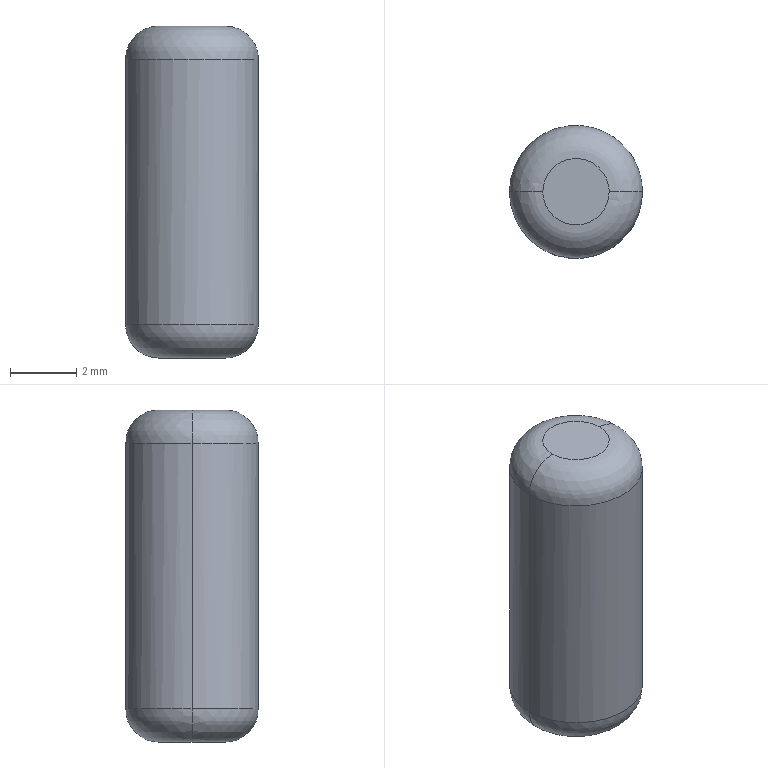Part | STEP file | CHOT DINH VI 4X10 | 1 solid | 8 faces | box 4 x 4 x 10 mm | volume 120.876 mm3 | spline 4 | cylinder 2 | plane 2 | commonest cylinder face diameters 4 x2
STEP:
#1=CARTESIAN_POINT('',(0.,0.,0.));
#2=DIRECTION('',(0.,0.,1.));
#3=DIRECTION('',(1.,0.,0.));
#4=AXIS2_PLACEMENT_3D('',#1,#2,#3);
#5=CARTESIAN_POINT('',(-2.,0.,1.));
#6=VERTEX_POINT('',#5);
#7=CARTESIAN_POINT('',(2.,0.,1.));
#8=VERTEX_POINT('',#7);
#9=CARTESIAN_POINT('',(-2.,0.,1.));
#10=CARTESIAN_POINT('',(-2.,-0.2618,1.));
#11=CARTESIAN_POINT('',(-1.948,-0.5235,1.));
#12=CARTESIAN_POINT('',(-1.748,-1.007,1.));
#13=CARTESIAN_POINT('',(-1.599,-1.229,1.));
#14=CARTESIAN_POINT('',(-1.229,-1.599,1.));
#15=CARTESIAN_POINT('',(-1.007,-1.748,1.));
#16=CARTESIAN_POINT('',(-0.5235,-1.948,1.));
#17=CARTESIAN_POINT('',(-0.2618,-2.,1.));
#18=CARTESIAN_POINT('',(0.2618,-2.,1.));
#19=CARTESIAN_POINT('',(0.5235,-1.948,1.));
#20=CARTESIAN_POINT('',(1.007,-1.748,1.));
#21=CARTESIAN_POINT('',(1.229,-1.599,1.));
#22=CARTESIAN_POINT('',(1.599,-1.229,1.));
#23=CARTESIAN_POINT('',(1.748,-1.007,1.));
#24=CARTESIAN_POINT('',(1.948,-0.5235,1.));
#25=CARTESIAN_POINT('',(2.,-0.2618,1.));
#26=CARTESIAN_POINT('',(2.,0.,1.));
#27=B_SPLINE_CURVE_WITH_KNOTS('',3,(#9,#10,#11,#12,#13,#14,#15,#16,#17,#18,#19,#20,#21,#22,#23,#24,#25,#26),.UNSPECIFIED.,.F.,.F.,(4,2,2,2,2,2,2,2,4),(0.5,0.5625,0.625,0.6875,0.75,0.8125,0.875,0.9375,1.),.UNSPECIFIED.);
#28=CARTESIAN_POINT('',(2.,0.,1.));
#29=CARTESIAN_POINT('',(2.,2.,1.));
#30=CARTESIAN_POINT('',(0.,2.,1.));
#31=CARTESIAN_POINT('',(-2.,2.,1.));
#32=CARTESIAN_POINT('',(-2.,0.,1.));
#33=CARTESIAN_POINT('',(-2.,-2.,1.));
#34=CARTESIAN_POINT('',(0.,-2.,1.));
#35=CARTESIAN_POINT('',(2.,-2.,1.));
#36=CARTESIAN_POINT('',(2.,0.,1.));
#37=CARTESIAN_POINT('',(2.,0.,0.));
#38=CARTESIAN_POINT('',(2.,2.,0.));
#39=CARTESIAN_POINT('',(0.,2.,0.));
#40=CARTESIAN_POINT('',(-2.,2.,0.));
#41=CARTESIAN_POINT('',(-2.,0.,0.));
#42=CARTESIAN_POINT('',(-2.,-2.,0.));
#43=CARTESIAN_POINT('',(0.,-2.,0.));
#44=CARTESIAN_POINT('',(2.,-2.,0.));
#45=CARTESIAN_POINT('',(2.,0.,0.));
#46=CARTESIAN_POINT('',(1.,0.,0.));
#47=CARTESIAN_POINT('',(1.,1.,0.));
#48=CARTESIAN_POINT('',(0.,1.,0.));
#49=CARTESIAN_POINT('',(-1.,1.,0.));
#50=CARTESIAN_POINT('',(-1.,0.,0.));
#51=CARTESIAN_POINT('',(-1.,-1.,0.));
#52=CARTESIAN_POINT('',(0.,-1.,0.));
#53=CARTESIAN_POINT('',(1.,-1.,0.));
#54=CARTESIAN_POINT('',(1.,0.,0.));
#55=(BOUNDED_SURFACE()B_SPLINE_SURFACE(2,2,((#28,#29,#30,#31,#32,#33,#34,#35,#36),(#37,#38,#39,#40,#41,#42,#43,#44,#45),(#46,#47,#48,#49,#50,#51,#52,#53,#54)),.UNSPECIFIED.,.F.,.T.,.F.)B_SPLINE_SURFACE_WITH_KNOTS((3,3),(1,2,2,2,2,2,1),(0.,1.571),(-1.571,0.,1.571,3.142,4.712,6.283,7.854),.UNSPECIFIED.)GEOMETRIC_REPRESENTATION_ITEM()RATIONAL_B_SPLINE_SURFACE(((1.,0.7071,1.,0.7071,1.,0.7071,1.,0.7071,1.),(0.7071,0.5,0.7071,0.5,0.7071,0.5,0.7071,0.5,0.7071),(1.,0.7071,1.,0.7071,1.,0.7071,1.,0.7071,1.)))REPRESENTATION_ITEM('')SURFACE());
#56=CARTESIAN_POINT('',(0.,3.142));
#57=CARTESIAN_POINT('',(0.,3.168));
#58=CARTESIAN_POINT('',(0.,3.22));
#59=CARTESIAN_POINT('',(0.,3.296));
#60=CARTESIAN_POINT('',(0.,3.37));
#61=CARTESIAN_POINT('',(0.,3.443));
#62=CARTESIAN_POINT('',(0.,3.515));
#63=CARTESIAN_POINT('',(0.,3.585));
#64=CARTESIAN_POINT('',(0.,3.654));
#65=CARTESIAN_POINT('',(0.,3.723));
#66=CARTESIAN_POINT('',(0.,3.791));
#67=CARTESIAN_POINT('',(0.,3.859));
#68=CARTESIAN_POINT('',(0.,3.927));
#69=CARTESIAN_POINT('',(0.,3.995));
#70=CARTESIAN_POINT('',(0.,4.063));
#71=CARTESIAN_POINT('',(0.,4.131));
#72=CARTESIAN_POINT('',(0.,4.199));
#73=CARTESIAN_POINT('',(0.,4.269));
#74=CARTESIAN_POINT('',(0.,4.339));
#75=CARTESIAN_POINT('',(0.,4.411));
#76=CARTESIAN_POINT('',(0.,4.483));
#77=CARTESIAN_POINT('',(0.,4.558));
#78=CARTESIAN_POINT('',(0.,4.634));
#79=CARTESIAN_POINT('',(0.,4.712));
#80=CARTESIAN_POINT('',(0.,4.791));
#81=CARTESIAN_POINT('',(0.,4.867));
#82=CARTESIAN_POINT('',(0.,4.941));
#83=CARTESIAN_POINT('',(0.,5.014));
#84=CARTESIAN_POINT('',(0.,5.085));
#85=CARTESIAN_POINT('',(0.,5.156));
#86=CARTESIAN_POINT('',(0.,5.225));
#87=CARTESIAN_POINT('',(0.,5.294));
#88=CARTESIAN_POINT('',(0.,5.362));
#89=CARTESIAN_POINT('',(0.,5.43));
#90=CARTESIAN_POINT('',(0.,5.498));
#91=CARTESIAN_POINT('',(0.,5.565));
#92=CARTESIAN_POINT('',(0.,5.633));
#93=CARTESIAN_POINT('',(0.,5.702));
#94=CARTESIAN_POINT('',(0.,5.77));
#95=CARTESIAN_POINT('',(0.,5.84));
#96=CARTESIAN_POINT('',(0.,5.91));
#97=CARTESIAN_POINT('',(0.,5.982));
#98=CARTESIAN_POINT('',(0.,6.054));
#99=CARTESIAN_POINT('',(0.,6.129));
#100=CARTESIAN_POINT('',(0.,6.205));
#101=CARTESIAN_POINT('',(0.,6.257));
#102=CARTESIAN_POINT('',(0.,6.283));
#103=B_SPLINE_CURVE_WITH_KNOTS('',3,(#56,#57,#58,#59,#60,#61,#62,#63,#64,#65,#66,#67,#68,#69,#70,#71,#72,#73,#74,#75,#76,#77,#78,#79,#80,#81,#82,#83,#84,#85,#86,#87,#88,#89,#90,#91,#92,#93,#94,#95,#96,#97,#98,#99,#100,#101,#102),.UNSPECIFIED.,.F.,.F.,(4,1,1,1,1,1,1,1,1,1,1,1,1,1,1,1,1,1,1,1,1,1,1,1,1,1,1,1,1,1,1,1,1,1,1,1,1,1,1,1,1,1,1,1,4),(0.5,0.5114,0.5227,0.5341,0.5455,0.5568,0.5682,0.5795,0.5909,0.6023,0.6136,0.625,0.6364,0.6477,0.6591,0.6705,0.6818,0.6932,0.7045,0.7159,0.7273,0.7386,0.75,0.7614,0.7727,0.7841,0.7955,0.8068,0.8182,0.8295,0.8409,0.8523,0.8636,0.875,0.8864,0.8977,0.9091,0.9205,0.9318,0.9432,0.9545,0.9659,0.9773,0.9886,1.),.QUASI_UNIFORM_KNOTS.);
#104=(GEOMETRIC_REPRESENTATION_CONTEXT(2)PARAMETRIC_REPRESENTATION_CONTEXT()REPRESENTATION_CONTEXT('',''));
#105=DEFINITIONAL_REPRESENTATION('',(#103),#104);
#106=PCURVE('',#55,#105);
#107=CARTESIAN_POINT('',(0.,0.,0.));
#108=DIRECTION('',(0.,0.,1.));
#109=DIRECTION('',(1.,0.,0.));
#110=AXIS2_PLACEMENT_3D('',#107,#108,#109);
#111=CYLINDRICAL_SURFACE('',#110,2.);
#112=CARTESIAN_POINT('',(3.142,1.));
#113=CARTESIAN_POINT('',(6.283,1.));
#114=B_SPLINE_CURVE_WITH_KNOTS('',1,(#112,#113),.UNSPECIFIED.,.F.,.F.,(2,2),(0.5,1.),.PIECEWISE_BEZIER_KNOTS.);
#115=(GEOMETRIC_REPRESENTATION_CONTEXT(2)PARAMETRIC_REPRESENTATION_CONTEXT()REPRESENTATION_CONTEXT('',''));
#116=DEFINITIONAL_REPRESENTATION('',(#114),#115);
#117=PCURVE('',#111,#116);
#118=SURFACE_CURVE('',#27,(#106,#117),.PCURVE_S1.);
#119=EDGE_CURVE('',#6,#8,#118,.T.);
#120=ORIENTED_EDGE('',*,*,#119,.F.);
#121=CARTESIAN_POINT('',(-1.,0.,0.));
#122=VERTEX_POINT('',#121);
#123=CARTESIAN_POINT('',(-2.,0.,1.));
#124=CARTESIAN_POINT('',(-2.,0.,0.));
#125=CARTESIAN_POINT('',(-1.,0.,0.));
#126=(BOUNDED_CURVE()B_SPLINE_CURVE(2,(#123,#124,#125),.UNSPECIFIED.,.F.,.F.)B_SPLINE_CURVE_WITH_KNOTS((3,3),(0.,1.571),.PIECEWISE_BEZIER_KNOTS.)CURVE()GEOMETRIC_REPRESENTATION_ITEM()RATIONAL_B_SPLINE_CURVE((1.,0.7071,1.))REPRESENTATION_ITEM(''));
#127=CARTESIAN_POINT('',(0.,3.142));
#128=DIRECTION('',(1.,0.));
#129=VECTOR('',#128,1.);
#130=LINE('',#127,#129);
#131=(GEOMETRIC_REPRESENTATION_CONTEXT(2)PARAMETRIC_REPRESENTATION_CONTEXT()REPRESENTATION_CONTEXT('',''));
#132=DEFINITIONAL_REPRESENTATION('',(#130),#131);
#133=PCURVE('',#55,#132);
#134=CARTESIAN_POINT('',(2.,0.,1.));
#135=CARTESIAN_POINT('',(2.,2.,1.));
#136=CARTESIAN_POINT('',(0.,2.,1.));
#137=CARTESIAN_POINT('',(-2.,2.,1.));
#138=CARTESIAN_POINT('',(-2.,0.,1.));
#139=CARTESIAN_POINT('',(-2.,-2.,1.));
#140=CARTESIAN_POINT('',(0.,-2.,1.));
#141=CARTESIAN_POINT('',(2.,-2.,1.));
#142=CARTESIAN_POINT('',(2.,0.,1.));
#143=CARTESIAN_POINT('',(2.,0.,0.));
#144=CARTESIAN_POINT('',(2.,2.,0.));
#145=CARTESIAN_POINT('',(0.,2.,0.));
#146=CARTESIAN_POINT('',(-2.,2.,0.));
#147=CARTESIAN_POINT('',(-2.,0.,0.));
#148=CARTESIAN_POINT('',(-2.,-2.,0.));
#149=CARTESIAN_POINT('',(0.,-2.,0.));
#150=CARTESIAN_POINT('',(2.,-2.,0.));
#151=CARTESIAN_POINT('',(2.,0.,0.));
#152=CARTESIAN_POINT('',(1.,0.,0.));
#153=CARTESIAN_POINT('',(1.,1.,0.));
#154=CARTESIAN_POINT('',(0.,1.,0.));
#155=CARTESIAN_POINT('',(-1.,1.,0.));
#156=CARTESIAN_POINT('',(-1.,0.,0.));
#157=CARTESIAN_POINT('',(-1.,-1.,0.));
#158=CARTESIAN_POINT('',(0.,-1.,0.));
#159=CARTESIAN_POINT('',(1.,-1.,0.));
#160=CARTESIAN_POINT('',(1.,0.,0.));
#161=(BOUNDED_SURFACE()B_SPLINE_SURFACE(2,2,((#134,#135,#136,#137,#138,#139,#140,#141,#142),(#143,#144,#145,#146,#147,#148,#149,#150,#151),(#152,#153,#154,#155,#156,#157,#158,#159,#160)),.UNSPECIFIED.,.F.,.T.,.F.)B_SPLINE_SURFACE_WITH_KNOTS((3,3),(1,2,2,2,2,2,1),(0.,1.571),(-1.571,0.,1.571,3.142,4.712,6.283,7.854),.UNSPECIFIED.)GEOMETRIC_REPRESENTATION_ITEM()RATIONAL_B_SPLINE_SURFACE(((1.,0.7071,1.,0.7071,1.,0.7071,1.,0.7071,1.),(0.7071,0.5,0.7071,0.5,0.7071,0.5,0.7071,0.5,0.7071),(1.,0.7071,1.,0.7071,1.,0.7071,1.,0.7071,1.)))REPRESENTATION_ITEM('')SURFACE());
#162=CARTESIAN_POINT('',(0.,3.142));
#163=DIRECTION('',(1.,0.));
#164=VECTOR('',#163,1.);
#165=LINE('',#162,#164);
#166=(GEOMETRIC_REPRESENTATION_CONTEXT(2)PARAMETRIC_REPRESENTATION_CONTEXT()REPRESENTATION_CONTEXT('',''));
#167=DEFINITIONAL_REPRESENTATION('',(#165),#166);
#168=PCURVE('',#161,#167);
#169=SURFACE_CURVE('',#126,(#133,#168),.PCURVE_S1.);
#170=EDGE_CURVE('',#6,#122,#169,.T.);
#171=ORIENTED_EDGE('',*,*,#170,.T.);
#172=CARTESIAN_POINT('',(1.,0.,0.));
#173=VERTEX_POINT('',#172);
#174=CARTESIAN_POINT('',(-1.,0.,0.));
#175=CARTESIAN_POINT('',(-1.,-1.,0.));
#176=CARTESIAN_POINT('',(0.,-1.,0.));
#177=CARTESIAN_POINT('',(1.,-1.,0.));
#178=CARTESIAN_POINT('',(1.,0.,0.));
#179=(BOUNDED_CURVE()B_SPLINE_CURVE(2,(#174,#175,#176,#177,#178),.UNSPECIFIED.,.F.,.F.)B_SPLINE_CURVE_WITH_KNOTS((3,2,3),(0.5,0.75,1.),.PIECEWISE_BEZIER_KNOTS.)CURVE()GEOMETRIC_REPRESENTATION_ITEM()RATIONAL_B_SPLINE_CURVE((1.,0.7071,1.,0.7071,1.))REPRESENTATION_ITEM(''));
#180=CARTESIAN_POINT('',(1.571,3.142));
#181=CARTESIAN_POINT('',(1.571,6.283));
#182=B_SPLINE_CURVE_WITH_KNOTS('',1,(#180,#181),.UNSPECIFIED.,.F.,.F.,(2,2),(0.5,1.),.PIECEWISE_BEZIER_KNOTS.);
#183=(GEOMETRIC_REPRESENTATION_CONTEXT(2)PARAMETRIC_REPRESENTATION_CONTEXT()REPRESENTATION_CONTEXT('',''));
#184=DEFINITIONAL_REPRESENTATION('',(#182),#183);
#185=PCURVE('',#55,#184);
#186=CARTESIAN_POINT('',(0.,0.,0.));
#187=DIRECTION('',(0.,0.,-1.));
#188=DIRECTION('',(-1.,0.,0.));
#189=AXIS2_PLACEMENT_3D('',#186,#187,#188);
#190=PLANE('',#189);
#191=CARTESIAN_POINT('',(1.,0.));
#192=CARTESIAN_POINT('',(1.,-1.));
#193=CARTESIAN_POINT('',(0.,-1.));
#194=CARTESIAN_POINT('',(-1.,-1.));
#195=CARTESIAN_POINT('',(-1.,0.));
#196=(BOUNDED_CURVE()B_SPLINE_CURVE(2,(#191,#192,#193,#194,#195),.UNSPECIFIED.,.F.,.F.)B_SPLINE_CURVE_WITH_KNOTS((3,2,3),(0.5,0.75,1.),.PIECEWISE_BEZIER_KNOTS.)CURVE()GEOMETRIC_REPRESENTATION_ITEM()RATIONAL_B_SPLINE_CURVE((1.,0.7071,1.,0.7071,1.))REPRESENTATION_ITEM(''));
#197=(GEOMETRIC_REPRESENTATION_CONTEXT(2)PARAMETRIC_REPRESENTATION_CONTEXT()REPRESENTATION_CONTEXT('',''));
#198=DEFINITIONAL_REPRESENTATION('',(#196),#197);
#199=PCURVE('',#190,#198);
#200=SURFACE_CURVE('',#179,(#185,#199),.PCURVE_S1.);
#201=EDGE_CURVE('',#122,#173,#200,.T.);
#202=ORIENTED_EDGE('',*,*,#201,.T.);
#203=CARTESIAN_POINT('',(2.,0.,1.));
#204=CARTESIAN_POINT('',(2.,0.,0.));
#205=CARTESIAN_POINT('',(1.,0.,0.));
#206=(BOUNDED_CURVE()B_SPLINE_CURVE(2,(#203,#204,#205),.UNSPECIFIED.,.F.,.F.)B_SPLINE_CURVE_WITH_KNOTS((3,3),(0.,1.571),.PIECEWISE_BEZIER_KNOTS.)CURVE()GEOMETRIC_REPRESENTATION_ITEM()RATIONAL_B_SPLINE_CURVE((1.,0.7071,1.))REPRESENTATION_ITEM(''));
#207=CARTESIAN_POINT('',(0.,6.283));
#208=DIRECTION('',(1.,0.));
#209=VECTOR('',#208,1.);
#210=LINE('',#207,#209);
#211=(GEOMETRIC_REPRESENTATION_CONTEXT(2)PARAMETRIC_REPRESENTATION_CONTEXT()REPRESENTATION_CONTEXT('',''));
#212=DEFINITIONAL_REPRESENTATION('',(#210),#211);
#213=PCURVE('',#55,#212);
#214=CARTESIAN_POINT('',(0.,0.));
#215=DIRECTION('',(1.,0.));
#216=VECTOR('',#215,1.);
#217=LINE('',#214,#216);
#218=(GEOMETRIC_REPRESENTATION_CONTEXT(2)PARAMETRIC_REPRESENTATION_CONTEXT()REPRESENTATION_CONTEXT('',''));
#219=DEFINITIONAL_REPRESENTATION('',(#217),#218);
#220=PCURVE('',#161,#219);
#221=SURFACE_CURVE('',#206,(#213,#220),.PCURVE_S1.);
#222=EDGE_CURVE('',#8,#173,#221,.T.);
#223=ORIENTED_EDGE('',*,*,#222,.F.);
#224=EDGE_LOOP('',(#120,#171,#202,#223));
#225=FACE_BOUND('',#224,.T.);
#226=ADVANCED_FACE('',(#225),#55,.T.);
#227=CARTESIAN_POINT('',(1.,0.,10.));
#228=VERTEX_POINT('',#227);
#229=CARTESIAN_POINT('',(-1.,0.,10.));
#230=VERTEX_POINT('',#229);
#231=CARTESIAN_POINT('',(1.,0.,10.));
#232=CARTESIAN_POINT('',(1.,-1.,10.));
#233=CARTESIAN_POINT('',(0.,-1.,10.));
#234=CARTESIAN_POINT('',(-1.,-1.,10.));
#235=CARTESIAN_POINT('',(-1.,0.,10.));
#236=(BOUNDED_CURVE()B_SPLINE_CURVE(2,(#231,#232,#233,#234,#235),.UNSPECIFIED.,.F.,.F.)B_SPLINE_CURVE_WITH_KNOTS((3,2,3),(0.,0.25,0.5),.PIECEWISE_BEZIER_KNOTS.)CURVE()GEOMETRIC_REPRESENTATION_ITEM()RATIONAL_B_SPLINE_CURVE((1.,0.7071,1.,0.7071,1.))REPRESENTATION_ITEM(''));
#237=CARTESIAN_POINT('',(1.,0.,10.));
#238=CARTESIAN_POINT('',(1.,1.,10.));
#239=CARTESIAN_POINT('',(0.,1.,10.));
#240=CARTESIAN_POINT('',(-1.,1.,10.));
#241=CARTESIAN_POINT('',(-1.,0.,10.));
#242=CARTESIAN_POINT('',(-1.,-1.,10.));
#243=CARTESIAN_POINT('',(0.,-1.,10.));
#244=CARTESIAN_POINT('',(1.,-1.,10.));
#245=CARTESIAN_POINT('',(1.,0.,10.));
#246=CARTESIAN_POINT('',(2.,0.,10.));
#247=CARTESIAN_POINT('',(2.,2.,10.));
#248=CARTESIAN_POINT('',(0.,2.,10.));
#249=CARTESIAN_POINT('',(-2.,2.,10.));
#250=CARTESIAN_POINT('',(-2.,0.,10.));
#251=CARTESIAN_POINT('',(-2.,-2.,10.));
#252=CARTESIAN_POINT('',(0.,-2.,10.));
#253=CARTESIAN_POINT('',(2.,-2.,10.));
#254=CARTESIAN_POINT('',(2.,0.,10.));
#255=CARTESIAN_POINT('',(2.,0.,9.));
#256=CARTESIAN_POINT('',(2.,2.,9.));
#257=CARTESIAN_POINT('',(0.,2.,9.));
#258=CARTESIAN_POINT('',(-2.,2.,9.));
#259=CARTESIAN_POINT('',(-2.,0.,9.));
#260=CARTESIAN_POINT('',(-2.,-2.,9.));
#261=CARTESIAN_POINT('',(0.,-2.,9.));
#262=CARTESIAN_POINT('',(2.,-2.,9.));
#263=CARTESIAN_POINT('',(2.,0.,9.));
#264=(BOUNDED_SURFACE()B_SPLINE_SURFACE(2,2,((#237,#238,#239,#240,#241,#242,#243,#244,#245),(#246,#247,#248,#249,#250,#251,#252,#253,#254),(#255,#256,#257,#258,#259,#260,#261,#262,#263)),.UNSPECIFIED.,.F.,.T.,.F.)B_SPLINE_SURFACE_WITH_KNOTS((3,3),(1,2,2,2,2,2,1),(-1.571,0.),(-1.571,0.,1.571,3.142,4.712,6.283,7.854),.UNSPECIFIED.)GEOMETRIC_REPRESENTATION_ITEM()RATIONAL_B_SPLINE_SURFACE(((1.,0.7071,1.,0.7071,1.,0.7071,1.,0.7071,1.),(0.7071,0.5,0.7071,0.5,0.7071,0.5,0.7071,0.5,0.7071),(1.,0.7071,1.,0.7071,1.,0.7071,1.,0.7071,1.)))REPRESENTATION_ITEM('')SURFACE());
#265=CARTESIAN_POINT('',(-1.571,6.283));
#266=CARTESIAN_POINT('',(-1.571,3.142));
#267=B_SPLINE_CURVE_WITH_KNOTS('',1,(#265,#266),.UNSPECIFIED.,.F.,.F.,(2,2),(0.,0.5),.PIECEWISE_BEZIER_KNOTS.);
#268=(GEOMETRIC_REPRESENTATION_CONTEXT(2)PARAMETRIC_REPRESENTATION_CONTEXT()REPRESENTATION_CONTEXT('',''));
#269=DEFINITIONAL_REPRESENTATION('',(#267),#268);
#270=PCURVE('',#264,#269);
#271=CARTESIAN_POINT('',(0.,0.,10.));
#272=DIRECTION('',(0.,0.,-1.));
#273=DIRECTION('',(-1.,0.,0.));
#274=AXIS2_PLACEMENT_3D('',#271,#272,#273);
#275=PLANE('',#274);
#276=CARTESIAN_POINT('',(-1.,0.));
#277=CARTESIAN_POINT('',(-1.,-1.));
#278=CARTESIAN_POINT('',(0.,-1.));
#279=CARTESIAN_POINT('',(1.,-1.));
#280=CARTESIAN_POINT('',(1.,0.));
#281=(BOUNDED_CURVE()B_SPLINE_CURVE(2,(#276,#277,#278,#279,#280),.UNSPECIFIED.,.F.,.F.)B_SPLINE_CURVE_WITH_KNOTS((3,2,3),(0.,0.25,0.5),.PIECEWISE_BEZIER_KNOTS.)CURVE()GEOMETRIC_REPRESENTATION_ITEM()RATIONAL_B_SPLINE_CURVE((1.,0.7071,1.,0.7071,1.))REPRESENTATION_ITEM(''));
#282=(GEOMETRIC_REPRESENTATION_CONTEXT(2)PARAMETRIC_REPRESENTATION_CONTEXT()REPRESENTATION_CONTEXT('',''));
#283=DEFINITIONAL_REPRESENTATION('',(#281),#282);
#284=PCURVE('',#275,#283);
#285=SURFACE_CURVE('',#236,(#270,#284),.PCURVE_S1.);
#286=EDGE_CURVE('',#228,#230,#285,.T.);
#287=ORIENTED_EDGE('',*,*,#286,.T.);
#288=CARTESIAN_POINT('',(-2.,0.,9.));
#289=VERTEX_POINT('',#288);
#290=CARTESIAN_POINT('',(-1.,0.,10.));
#291=CARTESIAN_POINT('',(-2.,0.,10.));
#292=CARTESIAN_POINT('',(-2.,0.,9.));
#293=(BOUNDED_CURVE()B_SPLINE_CURVE(2,(#290,#291,#292),.UNSPECIFIED.,.F.,.F.)B_SPLINE_CURVE_WITH_KNOTS((3,3),(-1.571,0.),.PIECEWISE_BEZIER_KNOTS.)CURVE()GEOMETRIC_REPRESENTATION_ITEM()RATIONAL_B_SPLINE_CURVE((1.,0.7071,1.))REPRESENTATION_ITEM(''));
#294=CARTESIAN_POINT('',(0.,3.142));
#295=DIRECTION('',(1.,0.));
#296=VECTOR('',#295,1.);
#297=LINE('',#294,#296);
#298=(GEOMETRIC_REPRESENTATION_CONTEXT(2)PARAMETRIC_REPRESENTATION_CONTEXT()REPRESENTATION_CONTEXT('',''));
#299=DEFINITIONAL_REPRESENTATION('',(#297),#298);
#300=PCURVE('',#264,#299);
#301=CARTESIAN_POINT('',(1.,0.,10.));
#302=CARTESIAN_POINT('',(1.,1.,10.));
#303=CARTESIAN_POINT('',(0.,1.,10.));
#304=CARTESIAN_POINT('',(-1.,1.,10.));
#305=CARTESIAN_POINT('',(-1.,0.,10.));
#306=CARTESIAN_POINT('',(-1.,-1.,10.));
#307=CARTESIAN_POINT('',(0.,-1.,10.));
#308=CARTESIAN_POINT('',(1.,-1.,10.));
#309=CARTESIAN_POINT('',(1.,0.,10.));
#310=CARTESIAN_POINT('',(2.,0.,10.));
#311=CARTESIAN_POINT('',(2.,2.,10.));
#312=CARTESIAN_POINT('',(0.,2.,10.));
#313=CARTESIAN_POINT('',(-2.,2.,10.));
#314=CARTESIAN_POINT('',(-2.,0.,10.));
#315=CARTESIAN_POINT('',(-2.,-2.,10.));
#316=CARTESIAN_POINT('',(0.,-2.,10.));
#317=CARTESIAN_POINT('',(2.,-2.,10.));
#318=CARTESIAN_POINT('',(2.,0.,10.));
#319=CARTESIAN_POINT('',(2.,0.,9.));
#320=CARTESIAN_POINT('',(2.,2.,9.));
#321=CARTESIAN_POINT('',(0.,2.,9.));
#322=CARTESIAN_POINT('',(-2.,2.,9.));
#323=CARTESIAN_POINT('',(-2.,0.,9.));
#324=CARTESIAN_POINT('',(-2.,-2.,9.));
#325=CARTESIAN_POINT('',(0.,-2.,9.));
#326=CARTESIAN_POINT('',(2.,-2.,9.));
#327=CARTESIAN_POINT('',(2.,0.,9.));
#328=(BOUNDED_SURFACE()B_SPLINE_SURFACE(2,2,((#301,#302,#303,#304,#305,#306,#307,#308,#309),(#310,#311,#312,#313,#314,#315,#316,#317,#318),(#319,#320,#321,#322,#323,#324,#325,#326,#327)),.UNSPECIFIED.,.F.,.T.,.F.)B_SPLINE_SURFACE_WITH_KNOTS((3,3),(1,2,2,2,2,2,1),(-1.571,0.),(-1.571,0.,1.571,3.142,4.712,6.283,7.854),.UNSPECIFIED.)GEOMETRIC_REPRESENTATION_ITEM()RATIONAL_B_SPLINE_SURFACE(((1.,0.7071,1.,0.7071,1.,0.7071,1.,0.7071,1.),(0.7071,0.5,0.7071,0.5,0.7071,0.5,0.7071,0.5,0.7071),(1.,0.7071,1.,0.7071,1.,0.7071,1.,0.7071,1.)))REPRESENTATION_ITEM('')SURFACE());
#329=CARTESIAN_POINT('',(0.,3.142));
#330=DIRECTION('',(1.,0.));
#331=VECTOR('',#330,1.);
#332=LINE('',#329,#331);
#333=(GEOMETRIC_REPRESENTATION_CONTEXT(2)PARAMETRIC_REPRESENTATION_CONTEXT()REPRESENTATION_CONTEXT('',''));
#334=DEFINITIONAL_REPRESENTATION('',(#332),#333);
#335=PCURVE('',#328,#334);
#336=SURFACE_CURVE('',#293,(#300,#335),.PCURVE_S1.);
#337=EDGE_CURVE('',#230,#289,#336,.T.);
#338=ORIENTED_EDGE('',*,*,#337,.T.);
#339=CARTESIAN_POINT('',(2.,0.,9.));
#340=VERTEX_POINT('',#339);
#341=CARTESIAN_POINT('',(2.,0.,9.));
#342=CARTESIAN_POINT('',(2.,-0.2618,9.));
#343=CARTESIAN_POINT('',(1.948,-0.5235,9.));
#344=CARTESIAN_POINT('',(1.748,-1.007,9.));
#345=CARTESIAN_POINT('',(1.599,-1.229,9.));
#346=CARTESIAN_POINT('',(1.229,-1.599,9.));
#347=CARTESIAN_POINT('',(1.007,-1.748,9.));
#348=CARTESIAN_POINT('',(0.5235,-1.948,9.));
#349=CARTESIAN_POINT('',(0.2618,-2.,9.));
#350=CARTESIAN_POINT('',(-0.2618,-2.,9.));
#351=CARTESIAN_POINT('',(-0.5235,-1.948,9.));
#352=CARTESIAN_POINT('',(-1.007,-1.748,9.));
#353=CARTESIAN_POINT('',(-1.229,-1.599,9.));
#354=CARTESIAN_POINT('',(-1.599,-1.229,9.));
#355=CARTESIAN_POINT('',(-1.748,-1.007,9.));
#356=CARTESIAN_POINT('',(-1.948,-0.5235,9.));
#357=CARTESIAN_POINT('',(-2.,-0.2618,9.));
#358=CARTESIAN_POINT('',(-2.,0.,9.));
#359=B_SPLINE_CURVE_WITH_KNOTS('',3,(#341,#342,#343,#344,#345,#346,#347,#348,#349,#350,#351,#352,#353,#354,#355,#356,#357,#358),.UNSPECIFIED.,.F.,.F.,(4,2,2,2,2,2,2,2,4),(0.,0.0625,0.125,0.1875,0.25,0.3125,0.375,0.4375,0.5),.UNSPECIFIED.);
#360=CARTESIAN_POINT('',(0.,6.283));
#361=CARTESIAN_POINT('',(0.,6.257));
#362=CARTESIAN_POINT('',(0.,6.205));
#363=CARTESIAN_POINT('',(0.,6.129));
#364=CARTESIAN_POINT('',(0.,6.054));
#365=CARTESIAN_POINT('',(0.,5.982));
#366=CARTESIAN_POINT('',(0.,5.91));
#367=CARTESIAN_POINT('',(0.,5.84));
#368=CARTESIAN_POINT('',(0.,5.77));
#369=CARTESIAN_POINT('',(0.,5.702));
#370=CARTESIAN_POINT('',(0.,5.633));
#371=CARTESIAN_POINT('',(0.,5.565));
#372=CARTESIAN_POINT('',(0.,5.498));
#373=CARTESIAN_POINT('',(0.,5.43));
#374=CARTESIAN_POINT('',(0.,5.362));
#375=CARTESIAN_POINT('',(0.,5.294));
#376=CARTESIAN_POINT('',(0.,5.225));
#377=CARTESIAN_POINT('',(0.,5.156));
#378=CARTESIAN_POINT('',(0.,5.085));
#379=CARTESIAN_POINT('',(0.,5.014));
#380=CARTESIAN_POINT('',(0.,4.941));
#381=CARTESIAN_POINT('',(0.,4.867));
#382=CARTESIAN_POINT('',(0.,4.791));
#383=CARTESIAN_POINT('',(0.,4.712));
#384=CARTESIAN_POINT('',(0.,4.634));
#385=CARTESIAN_POINT('',(0.,4.558));
#386=CARTESIAN_POINT('',(0.,4.483));
#387=CARTESIAN_POINT('',(0.,4.411));
#388=CARTESIAN_POINT('',(0.,4.339));
#389=CARTESIAN_POINT('',(0.,4.269));
#390=CARTESIAN_POINT('',(0.,4.199));
#391=CARTESIAN_POINT('',(0.,4.131));
#392=CARTESIAN_POINT('',(0.,4.063));
#393=CARTESIAN_POINT('',(0.,3.995));
#394=CARTESIAN_POINT('',(0.,3.927));
#395=CARTESIAN_POINT('',(0.,3.859));
#396=CARTESIAN_POINT('',(0.,3.791));
#397=CARTESIAN_POINT('',(0.,3.723));
#398=CARTESIAN_POINT('',(0.,3.654));
#399=CARTESIAN_POINT('',(0.,3.585));
#400=CARTESIAN_POINT('',(0.,3.515));
#401=CARTESIAN_POINT('',(0.,3.443));
#402=CARTESIAN_POINT('',(0.,3.37));
#403=CARTESIAN_POINT('',(0.,3.296));
#404=CARTESIAN_POINT('',(0.,3.22));
#405=CARTESIAN_POINT('',(0.,3.168));
#406=CARTESIAN_POINT('',(0.,3.142));
#407=B_SPLINE_CURVE_WITH_KNOTS('',3,(#360,#361,#362,#363,#364,#365,#366,#367,#368,#369,#370,#371,#372,#373,#374,#375,#376,#377,#378,#379,#380,#381,#382,#383,#384,#385,#386,#387,#388,#389,#390,#391,#392,#393,#394,#395,#396,#397,#398,#399,#400,#401,#402,#403,#404,#405,#406),.UNSPECIFIED.,.F.,.F.,(4,1,1,1,1,1,1,1,1,1,1,1,1,1,1,1,1,1,1,1,1,1,1,1,1,1,1,1,1,1,1,1,1,1,1,1,1,1,1,1,1,1,1,1,4),(0.,0.01136,0.02273,0.03409,0.04545,0.05682,0.06818,0.07955,0.09091,0.1023,0.1136,0.125,0.1364,0.1477,0.1591,0.1705,0.1818,0.1932,0.2045,0.2159,0.2273,0.2386,0.25,0.2614,0.2727,0.2841,0.2955,0.3068,0.3182,0.3295,0.3409,0.3523,0.3636,0.375,0.3864,0.3977,0.4091,0.4205,0.4318,0.4432,0.4545,0.4659,0.4773,0.4886,0.5),.QUASI_UNIFORM_KNOTS.);
#408=(GEOMETRIC_REPRESENTATION_CONTEXT(2)PARAMETRIC_REPRESENTATION_CONTEXT()REPRESENTATION_CONTEXT('',''));
#409=DEFINITIONAL_REPRESENTATION('',(#407),#408);
#410=PCURVE('',#264,#409);
#411=CARTESIAN_POINT('',(6.283,9.));
#412=CARTESIAN_POINT('',(3.142,9.));
#413=B_SPLINE_CURVE_WITH_KNOTS('',1,(#411,#412),.UNSPECIFIED.,.F.,.F.,(2,2),(0.,0.5),.PIECEWISE_BEZIER_KNOTS.);
#414=(GEOMETRIC_REPRESENTATION_CONTEXT(2)PARAMETRIC_REPRESENTATION_CONTEXT()REPRESENTATION_CONTEXT('',''));
#415=DEFINITIONAL_REPRESENTATION('',(#413),#414);
#416=PCURVE('',#111,#415);
#417=SURFACE_CURVE('',#359,(#410,#416),.PCURVE_S1.);
#418=EDGE_CURVE('',#340,#289,#417,.T.);
#419=ORIENTED_EDGE('',*,*,#418,.F.);
#420=CARTESIAN_POINT('',(1.,0.,10.));
#421=CARTESIAN_POINT('',(2.,0.,10.));
#422=CARTESIAN_POINT('',(2.,0.,9.));
#423=(BOUNDED_CURVE()B_SPLINE_CURVE(2,(#420,#421,#422),.UNSPECIFIED.,.F.,.F.)B_SPLINE_CURVE_WITH_KNOTS((3,3),(-1.571,0.),.PIECEWISE_BEZIER_KNOTS.)CURVE()GEOMETRIC_REPRESENTATION_ITEM()RATIONAL_B_SPLINE_CURVE((1.,0.7071,1.))REPRESENTATION_ITEM(''));
#424=CARTESIAN_POINT('',(0.,6.283));
#425=DIRECTION('',(1.,0.));
#426=VECTOR('',#425,1.);
#427=LINE('',#424,#426);
#428=(GEOMETRIC_REPRESENTATION_CONTEXT(2)PARAMETRIC_REPRESENTATION_CONTEXT()REPRESENTATION_CONTEXT('',''));
#429=DEFINITIONAL_REPRESENTATION('',(#427),#428);
#430=PCURVE('',#264,#429);
#431=CARTESIAN_POINT('',(0.,0.));
#432=DIRECTION('',(1.,0.));
#433=VECTOR('',#432,1.);
#434=LINE('',#431,#433);
#435=(GEOMETRIC_REPRESENTATION_CONTEXT(2)PARAMETRIC_REPRESENTATION_CONTEXT()REPRESENTATION_CONTEXT('',''));
#436=DEFINITIONAL_REPRESENTATION('',(#434),#435);
#437=PCURVE('',#328,#436);
#438=SURFACE_CURVE('',#423,(#430,#437),.PCURVE_S1.);
#439=EDGE_CURVE('',#228,#340,#438,.T.);
#440=ORIENTED_EDGE('',*,*,#439,.F.);
#441=EDGE_LOOP('',(#287,#338,#419,#440));
#442=FACE_BOUND('',#441,.T.);
#443=ADVANCED_FACE('',(#442),#264,.T.);
#444=CARTESIAN_POINT('',(2.,0.,1.));
#445=CARTESIAN_POINT('',(2.,0.2618,1.));
#446=CARTESIAN_POINT('',(1.948,0.5235,1.));
#447=CARTESIAN_POINT('',(1.748,1.007,1.));
#448=CARTESIAN_POINT('',(1.599,1.229,1.));
#449=CARTESIAN_POINT('',(1.229,1.599,1.));
#450=CARTESIAN_POINT('',(1.007,1.748,1.));
#451=CARTESIAN_POINT('',(0.5235,1.948,1.));
#452=CARTESIAN_POINT('',(0.2618,2.,1.));
#453=CARTESIAN_POINT('',(-0.2618,2.,1.));
#454=CARTESIAN_POINT('',(-0.5235,1.948,1.));
#455=CARTESIAN_POINT('',(-1.007,1.748,1.));
#456=CARTESIAN_POINT('',(-1.229,1.599,1.));
#457=CARTESIAN_POINT('',(-1.599,1.229,1.));
#458=CARTESIAN_POINT('',(-1.748,1.007,1.));
#459=CARTESIAN_POINT('',(-1.948,0.5235,1.));
#460=CARTESIAN_POINT('',(-2.,0.2618,1.));
#461=CARTESIAN_POINT('',(-2.,0.,1.));
#462=B_SPLINE_CURVE_WITH_KNOTS('',3,(#444,#445,#446,#447,#448,#449,#450,#451,#452,#453,#454,#455,#456,#457,#458,#459,#460,#461),.UNSPECIFIED.,.F.,.F.,(4,2,2,2,2,2,2,2,4),(0.,0.0625,0.125,0.1875,0.25,0.3125,0.375,0.4375,0.5),.UNSPECIFIED.);
#463=CARTESIAN_POINT('',(0.,0.,0.));
#464=DIRECTION('',(0.,0.,1.));
#465=DIRECTION('',(1.,0.,0.));
#466=AXIS2_PLACEMENT_3D('',#463,#464,#465);
#467=CYLINDRICAL_SURFACE('',#466,2.);
#468=CARTESIAN_POINT('',(0.,1.));
#469=CARTESIAN_POINT('',(3.142,1.));
#470=B_SPLINE_CURVE_WITH_KNOTS('',1,(#468,#469),.UNSPECIFIED.,.F.,.F.,(2,2),(0.,0.5),.PIECEWISE_BEZIER_KNOTS.);
#471=(GEOMETRIC_REPRESENTATION_CONTEXT(2)PARAMETRIC_REPRESENTATION_CONTEXT()REPRESENTATION_CONTEXT('',''));
#472=DEFINITIONAL_REPRESENTATION('',(#470),#471);
#473=PCURVE('',#467,#472);
#474=CARTESIAN_POINT('',(0.,0.));
#475=CARTESIAN_POINT('',(0.,0.02643));
#476=CARTESIAN_POINT('',(0.,0.07852));
#477=CARTESIAN_POINT('',(0.,0.1546));
#478=CARTESIAN_POINT('',(0.,0.2289));
#479=CARTESIAN_POINT('',(0.,0.3017));
#480=CARTESIAN_POINT('',(0.,0.3731));
#481=CARTESIAN_POINT('',(0.,0.4435));
#482=CARTESIAN_POINT('',(0.,0.5129));
#483=CARTESIAN_POINT('',(0.,0.5816));
#484=CARTESIAN_POINT('',(0.,0.6498));
#485=CARTESIAN_POINT('',(0.,0.7177));
#486=CARTESIAN_POINT('',(0.,0.7854));
#487=CARTESIAN_POINT('',(0.,0.8531));
#488=CARTESIAN_POINT('',(0.,0.921));
#489=CARTESIAN_POINT('',(0.,0.9892));
#490=CARTESIAN_POINT('',(0.,1.058));
#491=CARTESIAN_POINT('',(0.,1.127));
#492=CARTESIAN_POINT('',(0.,1.198));
#493=CARTESIAN_POINT('',(0.,1.269));
#494=CARTESIAN_POINT('',(0.,1.342));
#495=CARTESIAN_POINT('',(0.,1.416));
#496=CARTESIAN_POINT('',(0.,1.492));
#497=CARTESIAN_POINT('',(0.,1.571));
#498=CARTESIAN_POINT('',(0.,1.649));
#499=CARTESIAN_POINT('',(0.,1.725));
#500=CARTESIAN_POINT('',(0.,1.8));
#501=CARTESIAN_POINT('',(0.,1.872));
#502=CARTESIAN_POINT('',(0.,1.944));
#503=CARTESIAN_POINT('',(0.,2.014));
#504=CARTESIAN_POINT('',(0.,2.084));
#505=CARTESIAN_POINT('',(0.,2.152));
#506=CARTESIAN_POINT('',(0.,2.221));
#507=CARTESIAN_POINT('',(0.,2.289));
#508=CARTESIAN_POINT('',(0.,2.356));
#509=CARTESIAN_POINT('',(0.,2.424));
#510=CARTESIAN_POINT('',(0.,2.492));
#511=CARTESIAN_POINT('',(0.,2.56));
#512=CARTESIAN_POINT('',(0.,2.629));
#513=CARTESIAN_POINT('',(0.,2.698));
#514=CARTESIAN_POINT('',(0.,2.768));
#515=CARTESIAN_POINT('',(0.,2.84));
#516=CARTESIAN_POINT('',(0.,2.913));
#517=CARTESIAN_POINT('',(0.,2.987));
#518=CARTESIAN_POINT('',(0.,3.063));
#519=CARTESIAN_POINT('',(0.,3.115));
#520=CARTESIAN_POINT('',(0.,3.142));
#521=B_SPLINE_CURVE_WITH_KNOTS('',3,(#474,#475,#476,#477,#478,#479,#480,#481,#482,#483,#484,#485,#486,#487,#488,#489,#490,#491,#492,#493,#494,#495,#496,#497,#498,#499,#500,#501,#502,#503,#504,#505,#506,#507,#508,#509,#510,#511,#512,#513,#514,#515,#516,#517,#518,#519,#520),.UNSPECIFIED.,.F.,.F.,(4,1,1,1,1,1,1,1,1,1,1,1,1,1,1,1,1,1,1,1,1,1,1,1,1,1,1,1,1,1,1,1,1,1,1,1,1,1,1,1,1,1,1,1,4),(0.,0.01136,0.02273,0.03409,0.04545,0.05682,0.06818,0.07955,0.09091,0.1023,0.1136,0.125,0.1364,0.1477,0.1591,0.1705,0.1818,0.1932,0.2045,0.2159,0.2273,0.2386,0.25,0.2614,0.2727,0.2841,0.2955,0.3068,0.3182,0.3295,0.3409,0.3523,0.3636,0.375,0.3864,0.3977,0.4091,0.4205,0.4318,0.4432,0.4545,0.4659,0.4773,0.4886,0.5),.QUASI_UNIFORM_KNOTS.);
#522=(GEOMETRIC_REPRESENTATION_CONTEXT(2)PARAMETRIC_REPRESENTATION_CONTEXT()REPRESENTATION_CONTEXT('',''));
#523=DEFINITIONAL_REPRESENTATION('',(#521),#522);
#524=PCURVE('',#161,#523);
#525=SURFACE_CURVE('',#462,(#473,#524),.PCURVE_S1.);
#526=EDGE_CURVE('',#8,#6,#525,.T.);
#527=ORIENTED_EDGE('',*,*,#526,.T.);
#528=CARTESIAN_POINT('',(-2.,0.,0.));
#529=DIRECTION('',(0.,0.,1.));
#530=VECTOR('',#529,1.);
#531=LINE('',#528,#530);
#532=CARTESIAN_POINT('',(3.142,0.));
#533=DIRECTION('',(0.,1.));
#534=VECTOR('',#533,1.);
#535=LINE('',#532,#534);
#536=(GEOMETRIC_REPRESENTATION_CONTEXT(2)PARAMETRIC_REPRESENTATION_CONTEXT()REPRESENTATION_CONTEXT('',''));
#537=DEFINITIONAL_REPRESENTATION('',(#535),#536);
#538=PCURVE('',#467,#537);
#539=CARTESIAN_POINT('',(3.142,0.));
#540=DIRECTION('',(0.,1.));
#541=VECTOR('',#540,1.);
#542=LINE('',#539,#541);
#543=(GEOMETRIC_REPRESENTATION_CONTEXT(2)PARAMETRIC_REPRESENTATION_CONTEXT()REPRESENTATION_CONTEXT('',''));
#544=DEFINITIONAL_REPRESENTATION('',(#542),#543);
#545=PCURVE('',#111,#544);
#546=SURFACE_CURVE('',#531,(#538,#545),.PCURVE_S1.);
#547=EDGE_CURVE('',#6,#289,#546,.T.);
#548=ORIENTED_EDGE('',*,*,#547,.T.);
#549=CARTESIAN_POINT('',(-2.,0.,9.));
#550=CARTESIAN_POINT('',(-2.,0.2618,9.));
#551=CARTESIAN_POINT('',(-1.948,0.5235,9.));
#552=CARTESIAN_POINT('',(-1.748,1.007,9.));
#553=CARTESIAN_POINT('',(-1.599,1.229,9.));
#554=CARTESIAN_POINT('',(-1.229,1.599,9.));
#555=CARTESIAN_POINT('',(-1.007,1.748,9.));
#556=CARTESIAN_POINT('',(-0.5235,1.948,9.));
#557=CARTESIAN_POINT('',(-0.2618,2.,9.));
#558=CARTESIAN_POINT('',(0.2618,2.,9.));
#559=CARTESIAN_POINT('',(0.5235,1.948,9.));
#560=CARTESIAN_POINT('',(1.007,1.748,9.));
#561=CARTESIAN_POINT('',(1.229,1.599,9.));
#562=CARTESIAN_POINT('',(1.599,1.229,9.));
#563=CARTESIAN_POINT('',(1.748,1.007,9.));
#564=CARTESIAN_POINT('',(1.948,0.5235,9.));
#565=CARTESIAN_POINT('',(2.,0.2618,9.));
#566=CARTESIAN_POINT('',(2.,0.,9.));
#567=B_SPLINE_CURVE_WITH_KNOTS('',3,(#549,#550,#551,#552,#553,#554,#555,#556,#557,#558,#559,#560,#561,#562,#563,#564,#565,#566),.UNSPECIFIED.,.F.,.F.,(4,2,2,2,2,2,2,2,4),(0.5,0.5625,0.625,0.6875,0.75,0.8125,0.875,0.9375,1.),.UNSPECIFIED.);
#568=CARTESIAN_POINT('',(3.142,9.));
#569=CARTESIAN_POINT('',(0.,9.));
#570=B_SPLINE_CURVE_WITH_KNOTS('',1,(#568,#569),.UNSPECIFIED.,.F.,.F.,(2,2),(0.5,1.),.PIECEWISE_BEZIER_KNOTS.);
#571=(GEOMETRIC_REPRESENTATION_CONTEXT(2)PARAMETRIC_REPRESENTATION_CONTEXT()REPRESENTATION_CONTEXT('',''));
#572=DEFINITIONAL_REPRESENTATION('',(#570),#571);
#573=PCURVE('',#467,#572);
#574=CARTESIAN_POINT('',(0.,3.142));
#575=CARTESIAN_POINT('',(0.,3.115));
#576=CARTESIAN_POINT('',(0.,3.063));
#577=CARTESIAN_POINT('',(0.,2.987));
#578=CARTESIAN_POINT('',(0.,2.913));
#579=CARTESIAN_POINT('',(0.,2.84));
#580=CARTESIAN_POINT('',(0.,2.768));
#581=CARTESIAN_POINT('',(0.,2.698));
#582=CARTESIAN_POINT('',(0.,2.629));
#583=CARTESIAN_POINT('',(0.,2.56));
#584=CARTESIAN_POINT('',(0.,2.492));
#585=CARTESIAN_POINT('',(0.,2.424));
#586=CARTESIAN_POINT('',(0.,2.356));
#587=CARTESIAN_POINT('',(0.,2.289));
#588=CARTESIAN_POINT('',(0.,2.221));
#589=CARTESIAN_POINT('',(0.,2.152));
#590=CARTESIAN_POINT('',(0.,2.084));
#591=CARTESIAN_POINT('',(0.,2.014));
#592=CARTESIAN_POINT('',(0.,1.944));
#593=CARTESIAN_POINT('',(0.,1.872));
#594=CARTESIAN_POINT('',(0.,1.8));
#595=CARTESIAN_POINT('',(0.,1.725));
#596=CARTESIAN_POINT('',(0.,1.649));
#597=CARTESIAN_POINT('',(0.,1.571));
#598=CARTESIAN_POINT('',(0.,1.492));
#599=CARTESIAN_POINT('',(0.,1.416));
#600=CARTESIAN_POINT('',(0.,1.342));
#601=CARTESIAN_POINT('',(0.,1.269));
#602=CARTESIAN_POINT('',(0.,1.198));
#603=CARTESIAN_POINT('',(0.,1.127));
#604=CARTESIAN_POINT('',(0.,1.058));
#605=CARTESIAN_POINT('',(0.,0.9892));
#606=CARTESIAN_POINT('',(0.,0.921));
#607=CARTESIAN_POINT('',(0.,0.8531));
#608=CARTESIAN_POINT('',(0.,0.7854));
#609=CARTESIAN_POINT('',(0.,0.7177));
#610=CARTESIAN_POINT('',(0.,0.6498));
#611=CARTESIAN_POINT('',(0.,0.5816));
#612=CARTESIAN_POINT('',(0.,0.5129));
#613=CARTESIAN_POINT('',(0.,0.4435));
#614=CARTESIAN_POINT('',(0.,0.3731));
#615=CARTESIAN_POINT('',(0.,0.3017));
#616=CARTESIAN_POINT('',(0.,0.2289));
#617=CARTESIAN_POINT('',(0.,0.1546));
#618=CARTESIAN_POINT('',(0.,0.07852));
#619=CARTESIAN_POINT('',(0.,0.02643));
#620=CARTESIAN_POINT('',(0.,0.));
#621=B_SPLINE_CURVE_WITH_KNOTS('',3,(#574,#575,#576,#577,#578,#579,#580,#581,#582,#583,#584,#585,#586,#587,#588,#589,#590,#591,#592,#593,#594,#595,#596,#597,#598,#599,#600,#601,#602,#603,#604,#605,#606,#607,#608,#609,#610,#611,#612,#613,#614,#615,#616,#617,#618,#619,#620),.UNSPECIFIED.,.F.,.F.,(4,1,1,1,1,1,1,1,1,1,1,1,1,1,1,1,1,1,1,1,1,1,1,1,1,1,1,1,1,1,1,1,1,1,1,1,1,1,1,1,1,1,1,1,4),(0.5,0.5114,0.5227,0.5341,0.5455,0.5568,0.5682,0.5795,0.5909,0.6023,0.6136,0.625,0.6364,0.6477,0.6591,0.6705,0.6818,0.6932,0.7045,0.7159,0.7273,0.7386,0.75,0.7614,0.7727,0.7841,0.7955,0.8068,0.8182,0.8295,0.8409,0.8523,0.8636,0.875,0.8864,0.8977,0.9091,0.9205,0.9318,0.9432,0.9545,0.9659,0.9773,0.9886,1.),.QUASI_UNIFORM_KNOTS.);
#622=(GEOMETRIC_REPRESENTATION_CONTEXT(2)PARAMETRIC_REPRESENTATION_CONTEXT()REPRESENTATION_CONTEXT('',''));
#623=DEFINITIONAL_REPRESENTATION('',(#621),#622);
#624=PCURVE('',#328,#623);
#625=SURFACE_CURVE('',#567,(#573,#624),.PCURVE_S1.);
#626=EDGE_CURVE('',#289,#340,#625,.T.);
#627=ORIENTED_EDGE('',*,*,#626,.T.);
#628=CARTESIAN_POINT('',(2.,0.,0.));
#629=DIRECTION('',(0.,0.,1.));
#630=VECTOR('',#629,1.);
#631=LINE('',#628,#630);
#632=CARTESIAN_POINT('',(0.,0.));
#633=DIRECTION('',(0.,1.));
#634=VECTOR('',#633,1.);
#635=LINE('',#632,#634);
#636=(GEOMETRIC_REPRESENTATION_CONTEXT(2)PARAMETRIC_REPRESENTATION_CONTEXT()REPRESENTATION_CONTEXT('',''));
#637=DEFINITIONAL_REPRESENTATION('',(#635),#636);
#638=PCURVE('',#467,#637);
#639=CARTESIAN_POINT('',(6.283,0.));
#640=DIRECTION('',(0.,1.));
#641=VECTOR('',#640,1.);
#642=LINE('',#639,#641);
#643=(GEOMETRIC_REPRESENTATION_CONTEXT(2)PARAMETRIC_REPRESENTATION_CONTEXT()REPRESENTATION_CONTEXT('',''));
#644=DEFINITIONAL_REPRESENTATION('',(#642),#643);
#645=PCURVE('',#111,#644);
#646=SURFACE_CURVE('',#631,(#638,#645),.PCURVE_S1.);
#647=EDGE_CURVE('',#8,#340,#646,.T.);
#648=ORIENTED_EDGE('',*,*,#647,.F.);
#649=EDGE_LOOP('',(#527,#548,#627,#648));
#650=FACE_BOUND('',#649,.T.);
#651=ADVANCED_FACE('',(#650),#467,.T.);
#652=ORIENTED_EDGE('',*,*,#547,.F.);
#653=ORIENTED_EDGE('',*,*,#119,.T.);
#654=ORIENTED_EDGE('',*,*,#647,.T.);
#655=ORIENTED_EDGE('',*,*,#418,.T.);
#656=EDGE_LOOP('',(#652,#653,#654,#655));
#657=FACE_BOUND('',#656,.T.);
#658=ADVANCED_FACE('',(#657),#111,.T.);
#659=ORIENTED_EDGE('',*,*,#170,.F.);
#660=ORIENTED_EDGE('',*,*,#526,.F.);
#661=ORIENTED_EDGE('',*,*,#222,.T.);
#662=CARTESIAN_POINT('',(1.,0.,0.));
#663=CARTESIAN_POINT('',(1.,1.,0.));
#664=CARTESIAN_POINT('',(0.,1.,0.));
#665=CARTESIAN_POINT('',(-1.,1.,0.));
#666=CARTESIAN_POINT('',(-1.,0.,0.));
#667=(BOUNDED_CURVE()B_SPLINE_CURVE(2,(#662,#663,#664,#665,#666),.UNSPECIFIED.,.F.,.F.)B_SPLINE_CURVE_WITH_KNOTS((3,2,3),(0.,0.25,0.5),.PIECEWISE_BEZIER_KNOTS.)CURVE()GEOMETRIC_REPRESENTATION_ITEM()RATIONAL_B_SPLINE_CURVE((1.,0.7071,1.,0.7071,1.))REPRESENTATION_ITEM(''));
#668=CARTESIAN_POINT('',(1.571,0.));
#669=CARTESIAN_POINT('',(1.571,3.142));
#670=B_SPLINE_CURVE_WITH_KNOTS('',1,(#668,#669),.UNSPECIFIED.,.F.,.F.,(2,2),(0.,0.5),.PIECEWISE_BEZIER_KNOTS.);
#671=(GEOMETRIC_REPRESENTATION_CONTEXT(2)PARAMETRIC_REPRESENTATION_CONTEXT()REPRESENTATION_CONTEXT('',''));
#672=DEFINITIONAL_REPRESENTATION('',(#670),#671);
#673=PCURVE('',#161,#672);
#674=CARTESIAN_POINT('',(-1.,0.));
#675=CARTESIAN_POINT('',(-1.,1.));
#676=CARTESIAN_POINT('',(0.,1.));
#677=CARTESIAN_POINT('',(1.,1.));
#678=CARTESIAN_POINT('',(1.,0.));
#679=(BOUNDED_CURVE()B_SPLINE_CURVE(2,(#674,#675,#676,#677,#678),.UNSPECIFIED.,.F.,.F.)B_SPLINE_CURVE_WITH_KNOTS((3,2,3),(0.,0.25,0.5),.PIECEWISE_BEZIER_KNOTS.)CURVE()GEOMETRIC_REPRESENTATION_ITEM()RATIONAL_B_SPLINE_CURVE((1.,0.7071,1.,0.7071,1.))REPRESENTATION_ITEM(''));
#680=(GEOMETRIC_REPRESENTATION_CONTEXT(2)PARAMETRIC_REPRESENTATION_CONTEXT()REPRESENTATION_CONTEXT('',''));
#681=DEFINITIONAL_REPRESENTATION('',(#679),#680);
#682=PCURVE('',#190,#681);
#683=SURFACE_CURVE('',#667,(#673,#682),.PCURVE_S1.);
#684=EDGE_CURVE('',#173,#122,#683,.T.);
#685=ORIENTED_EDGE('',*,*,#684,.T.);
#686=EDGE_LOOP('',(#659,#660,#661,#685));
#687=FACE_BOUND('',#686,.T.);
#688=ADVANCED_FACE('',(#687),#161,.T.);
#689=ORIENTED_EDGE('',*,*,#337,.F.);
#690=CARTESIAN_POINT('',(-1.,0.,10.));
#691=CARTESIAN_POINT('',(-1.,1.,10.));
#692=CARTESIAN_POINT('',(0.,1.,10.));
#693=CARTESIAN_POINT('',(1.,1.,10.));
#694=CARTESIAN_POINT('',(1.,0.,10.));
#695=(BOUNDED_CURVE()B_SPLINE_CURVE(2,(#690,#691,#692,#693,#694),.UNSPECIFIED.,.F.,.F.)B_SPLINE_CURVE_WITH_KNOTS((3,2,3),(0.5,0.75,1.),.PIECEWISE_BEZIER_KNOTS.)CURVE()GEOMETRIC_REPRESENTATION_ITEM()RATIONAL_B_SPLINE_CURVE((1.,0.7071,1.,0.7071,1.))REPRESENTATION_ITEM(''));
#696=CARTESIAN_POINT('',(-1.571,3.142));
#697=CARTESIAN_POINT('',(-1.571,0.));
#698=B_SPLINE_CURVE_WITH_KNOTS('',1,(#696,#697),.UNSPECIFIED.,.F.,.F.,(2,2),(0.5,1.),.PIECEWISE_BEZIER_KNOTS.);
#699=(GEOMETRIC_REPRESENTATION_CONTEXT(2)PARAMETRIC_REPRESENTATION_CONTEXT()REPRESENTATION_CONTEXT('',''));
#700=DEFINITIONAL_REPRESENTATION('',(#698),#699);
#701=PCURVE('',#328,#700);
#702=CARTESIAN_POINT('',(1.,0.));
#703=CARTESIAN_POINT('',(1.,1.));
#704=CARTESIAN_POINT('',(0.,1.));
#705=CARTESIAN_POINT('',(-1.,1.));
#706=CARTESIAN_POINT('',(-1.,0.));
#707=(BOUNDED_CURVE()B_SPLINE_CURVE(2,(#702,#703,#704,#705,#706),.UNSPECIFIED.,.F.,.F.)B_SPLINE_CURVE_WITH_KNOTS((3,2,3),(0.5,0.75,1.),.PIECEWISE_BEZIER_KNOTS.)CURVE()GEOMETRIC_REPRESENTATION_ITEM()RATIONAL_B_SPLINE_CURVE((1.,0.7071,1.,0.7071,1.))REPRESENTATION_ITEM(''));
#708=(GEOMETRIC_REPRESENTATION_CONTEXT(2)PARAMETRIC_REPRESENTATION_CONTEXT()REPRESENTATION_CONTEXT('',''));
#709=DEFINITIONAL_REPRESENTATION('',(#707),#708);
#710=PCURVE('',#275,#709);
#711=SURFACE_CURVE('',#695,(#701,#710),.PCURVE_S1.);
#712=EDGE_CURVE('',#230,#228,#711,.T.);
#713=ORIENTED_EDGE('',*,*,#712,.T.);
#714=ORIENTED_EDGE('',*,*,#439,.T.);
#715=ORIENTED_EDGE('',*,*,#626,.F.);
#716=EDGE_LOOP('',(#689,#713,#714,#715));
#717=FACE_BOUND('',#716,.T.);
#718=ADVANCED_FACE('',(#717),#328,.T.);
#719=ORIENTED_EDGE('',*,*,#684,.F.);
#720=ORIENTED_EDGE('',*,*,#201,.F.);
#721=EDGE_LOOP('',(#719,#720));
#722=FACE_BOUND('',#721,.T.);
#723=ADVANCED_FACE('',(#722),#190,.T.);
#724=ORIENTED_EDGE('',*,*,#286,.F.);
#725=ORIENTED_EDGE('',*,*,#712,.F.);
#726=EDGE_LOOP('',(#724,#725));
#727=FACE_BOUND('',#726,.T.);
#728=ADVANCED_FACE('',(#727),#275,.F.);
#729=CLOSED_SHELL('',(#226,#443,#651,#658,#688,#718,#723,#728));
#730=MANIFOLD_SOLID_BREP('',#729);
#731=(LENGTH_UNIT()NAMED_UNIT(*)SI_UNIT(.MILLI.,.METRE.));
#732=UNCERTAINTY_MEASURE_WITH_UNIT(LENGTH_MEASURE(0.00005),#731,'','');
#733=(NAMED_UNIT(*)PLANE_ANGLE_UNIT()SI_UNIT($,.RADIAN.));
#734=(NAMED_UNIT(*)SI_UNIT($,.STERADIAN.)SOLID_ANGLE_UNIT());
#735=(GEOMETRIC_REPRESENTATION_CONTEXT(3)GLOBAL_UNCERTAINTY_ASSIGNED_CONTEXT((#732))GLOBAL_UNIT_ASSIGNED_CONTEXT((#731,#733,#734))REPRESENTATION_CONTEXT('',''));
#736=ADVANCED_BREP_SHAPE_REPRESENTATION('',(#4,#730),#735);